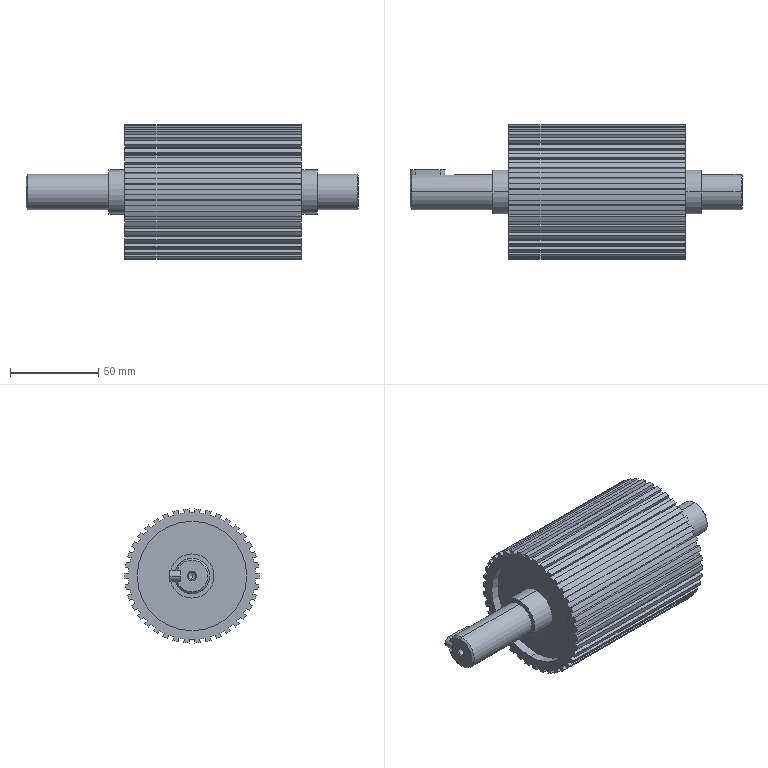Part | SolidWorks | 3 solids | 213 faces | box 188 x 76 x 75.929 mm | volume 254604 mm3 | cylinder 104 | plane 95 | cone 13 | spline 1 | commonest cylinder face diameters 72 x39 76 x38 62 x8 25 x6 4.2 x4 20 x4